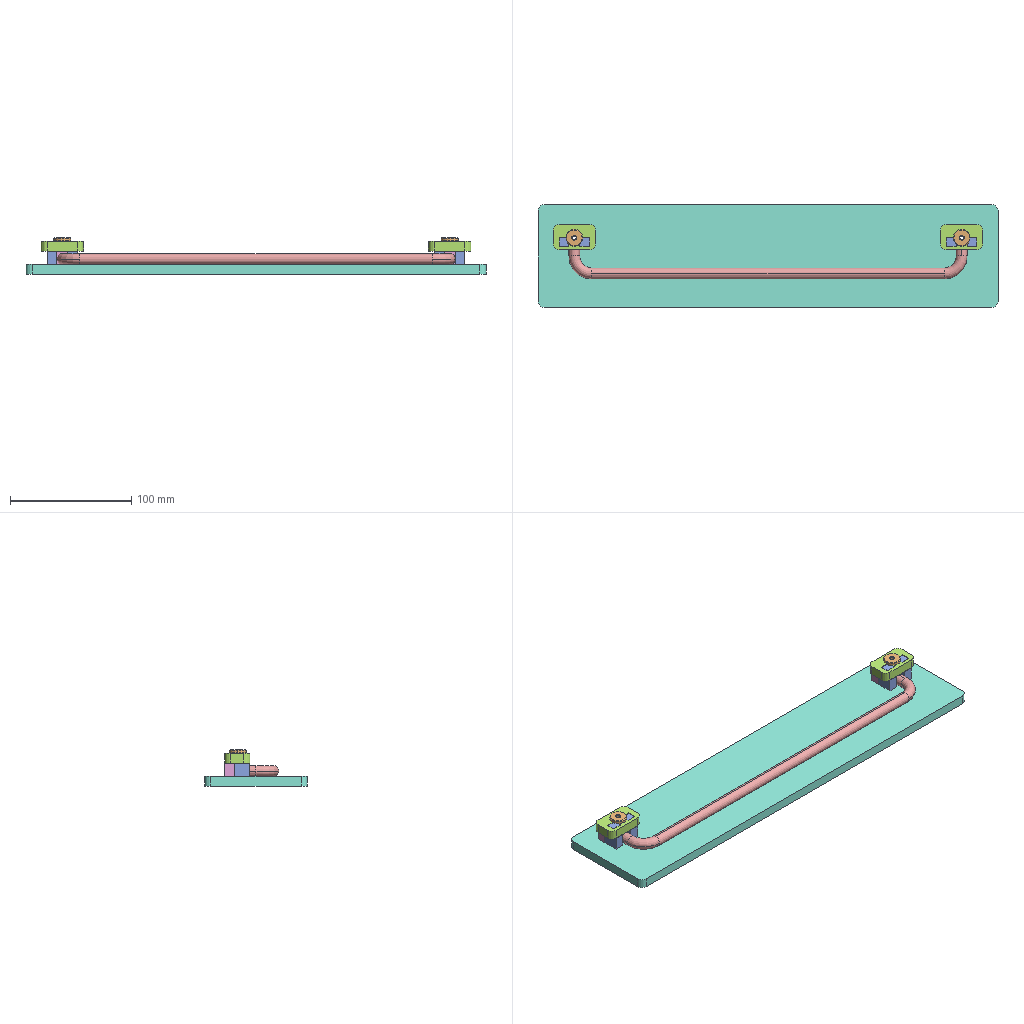Assembly | SolidWorks | 6 different items | 12 placed | box 380 x 85 x 30 mm
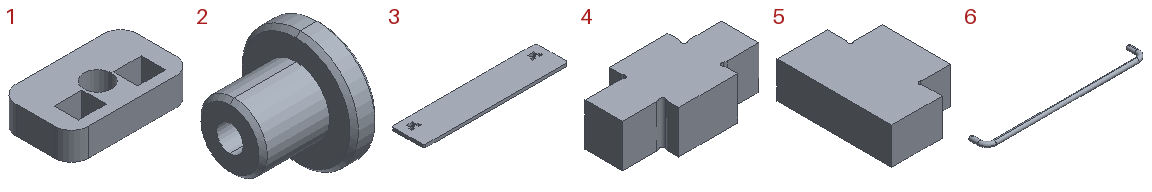Parts list (item | quantity | size | volume | features):
1 | x2 | 35.1 x 21 x 8 mm | 4427 mm3 | features Fillet 1, FlatPattern 1, SMBaseFlange 1, SheetMetal 1
2 | x2 | 11 x 14 x 14 mm | 760.339 mm3 | features Chamfer 1, Revolution 1
3 | x1 | 380 x 85 x 8 mm | 254362 mm3 | features Fillet 1, FlatPattern 1, SMBaseFlange 1, SheetMetal 1
4 | x4 | 25.5 x 13 x 8 mm | 1946 mm3 | features Fillet 1, FlatPattern 1, ICE 1, SMBaseFlange 1, SheetMetal 1
5 | x2 | 18 x 25.1 x 8 mm | 3044 mm3 | features Fillet 1, FlatPattern 1, ICE 1, SMBaseFlange 1, SheetMetal 1
6 | x1 | 329 x 37 x 9 mm | 23569 mm3 | features Chamfer 1, ICE 1, Sweep 1
Mates (type | each side: item.copy, entity, surface, feature):
InPlace | 4.1 plane | assembly plane
InPlace | 4.2 face plane Base-Flange1 | 1.1 plane
InPlace | 4.1 face plane Base-Flange1 | 5.1 plane
InPlace | 4.1 face plane Base-Flange1 | 3.1 plane
InPlace | 2.1 plane | assembly plane